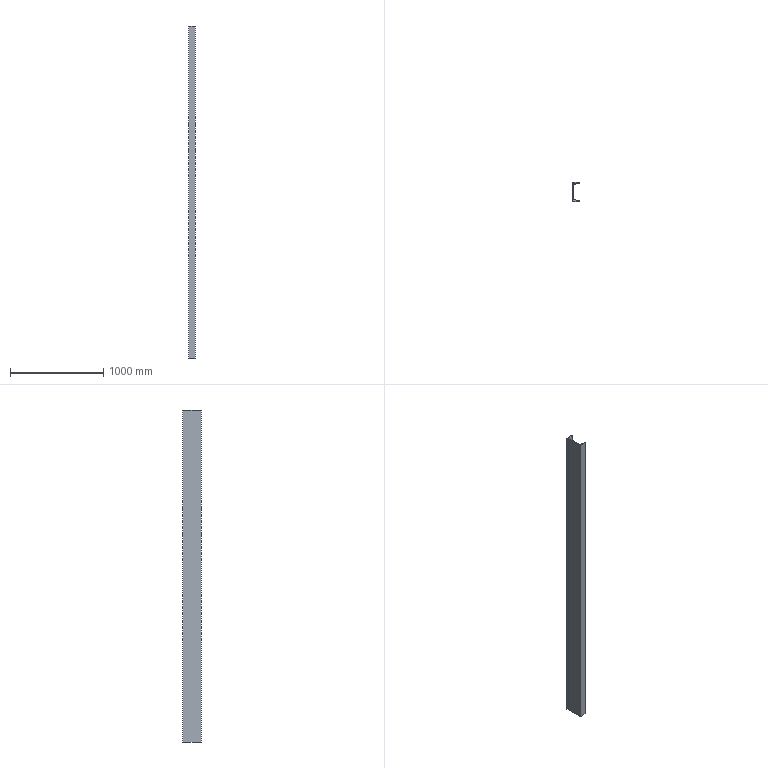Part | SolidWorks | features Extrusion 1 | 1 solid | 14 faces | box 73 x 200 x 3556 mm | volume 10184198 mm3 | plane 10 | cylinder 4 | commonest cylinder face diameters 11 x2 22 x2
STEP:
#1=CARTESIAN_POINT('',(73.,200.,-1778.));
#2=VERTEX_POINT('',#1);
#3=CARTESIAN_POINT('',(0.,200.,-1778.));
#4=VERTEX_POINT('',#3);
#5=CARTESIAN_POINT('',(0.,200.,-1778.));
#6=DIRECTION('',(-1.,0.,0.));
#7=VECTOR('',#6,1000.);
#8=LINE('',#5,#7);
#9=EDGE_CURVE('',#2,#4,#8,.T.);
#10=ORIENTED_EDGE('',*,*,#9,.T.);
#11=CARTESIAN_POINT('',(0.,200.,1778.));
#12=VERTEX_POINT('',#11);
#13=CARTESIAN_POINT('',(0.,200.,1778.));
#14=DIRECTION('',(0.,0.,-1.));
#15=VECTOR('',#14,1000.);
#16=LINE('',#13,#15);
#17=EDGE_CURVE('',#12,#4,#16,.T.);
#18=ORIENTED_EDGE('',*,*,#17,.F.);
#19=CARTESIAN_POINT('',(73.,200.,1778.));
#20=VERTEX_POINT('',#19);
#21=CARTESIAN_POINT('',(0.,200.,1778.));
#22=DIRECTION('',(-1.,0.,0.));
#23=VECTOR('',#22,1000.);
#24=LINE('',#21,#23);
#25=EDGE_CURVE('',#20,#12,#24,.T.);
#26=ORIENTED_EDGE('',*,*,#25,.F.);
#27=CARTESIAN_POINT('',(73.,200.,1778.));
#28=DIRECTION('',(0.,0.,-1.));
#29=VECTOR('',#28,1000.);
#30=LINE('',#27,#29);
#31=EDGE_CURVE('',#20,#2,#30,.T.);
#32=ORIENTED_EDGE('',*,*,#31,.T.);
#33=EDGE_LOOP('',(#10,#18,#26,#32));
#34=FACE_OUTER_BOUND('',#33,.T.);
#35=CARTESIAN_POINT('',(0.,200.,1778.));
#36=DIRECTION('',(0.,-1.,0.));
#37=DIRECTION('',(0.,0.,-1.));
#38=AXIS2_PLACEMENT_3D('',#35,#36,#37);
#39=PLANE('',#38);
#40=ADVANCED_FACE('',(#34),#39,.F.);
#41=CARTESIAN_POINT('',(0.,0.,-1778.));
#42=VERTEX_POINT('',#41);
#43=CARTESIAN_POINT('',(0.,0.,-1778.));
#44=DIRECTION('',(0.,-1.,0.));
#45=VECTOR('',#44,1000.);
#46=LINE('',#43,#45);
#47=EDGE_CURVE('',#4,#42,#46,.T.);
#48=ORIENTED_EDGE('',*,*,#47,.T.);
#49=CARTESIAN_POINT('',(0.,0.,1778.));
#50=VERTEX_POINT('',#49);
#51=CARTESIAN_POINT('',(0.,0.,1778.));
#52=DIRECTION('',(0.,0.,-1.));
#53=VECTOR('',#52,1000.);
#54=LINE('',#51,#53);
#55=EDGE_CURVE('',#50,#42,#54,.T.);
#56=ORIENTED_EDGE('',*,*,#55,.F.);
#57=CARTESIAN_POINT('',(0.,0.,1778.));
#58=DIRECTION('',(0.,-1.,0.));
#59=VECTOR('',#58,1000.);
#60=LINE('',#57,#59);
#61=EDGE_CURVE('',#12,#50,#60,.T.);
#62=ORIENTED_EDGE('',*,*,#61,.F.);
#63=ORIENTED_EDGE('',*,*,#17,.T.);
#64=EDGE_LOOP('',(#48,#56,#62,#63));
#65=FACE_OUTER_BOUND('',#64,.T.);
#66=CARTESIAN_POINT('',(0.,0.,1778.));
#67=DIRECTION('',(1.,0.,0.));
#68=DIRECTION('',(0.,0.,-1.));
#69=AXIS2_PLACEMENT_3D('',#66,#67,#68);
#70=PLANE('',#69);
#71=ADVANCED_FACE('',(#65),#70,.F.);
#72=CARTESIAN_POINT('',(73.,0.,-1778.));
#73=VERTEX_POINT('',#72);
#74=CARTESIAN_POINT('',(0.,0.,-1778.));
#75=DIRECTION('',(1.,0.,0.));
#76=VECTOR('',#75,1000.);
#77=LINE('',#74,#76);
#78=EDGE_CURVE('',#42,#73,#77,.T.);
#79=ORIENTED_EDGE('',*,*,#78,.T.);
#80=CARTESIAN_POINT('',(73.,0.,1778.));
#81=VERTEX_POINT('',#80);
#82=CARTESIAN_POINT('',(73.,0.,1778.));
#83=DIRECTION('',(0.,0.,-1.));
#84=VECTOR('',#83,1000.);
#85=LINE('',#82,#84);
#86=EDGE_CURVE('',#81,#73,#85,.T.);
#87=ORIENTED_EDGE('',*,*,#86,.F.);
#88=CARTESIAN_POINT('',(0.,0.,1778.));
#89=DIRECTION('',(1.,0.,0.));
#90=VECTOR('',#89,1000.);
#91=LINE('',#88,#90);
#92=EDGE_CURVE('',#50,#81,#91,.T.);
#93=ORIENTED_EDGE('',*,*,#92,.F.);
#94=ORIENTED_EDGE('',*,*,#55,.T.);
#95=EDGE_LOOP('',(#79,#87,#93,#94));
#96=FACE_OUTER_BOUND('',#95,.T.);
#97=CARTESIAN_POINT('',(0.,0.,1778.));
#98=DIRECTION('',(0.,1.,0.));
#99=DIRECTION('',(0.,0.,1.));
#100=AXIS2_PLACEMENT_3D('',#97,#98,#99);
#101=PLANE('',#100);
#102=ADVANCED_FACE('',(#96),#101,.F.);
#103=CARTESIAN_POINT('',(73.,3.967,-1778.));
#104=VERTEX_POINT('',#103);
#105=CARTESIAN_POINT('',(73.,3.967,-1778.));
#106=DIRECTION('',(0.,1.,0.));
#107=VECTOR('',#106,1000.);
#108=LINE('',#105,#107);
#109=EDGE_CURVE('',#73,#104,#108,.T.);
#110=ORIENTED_EDGE('',*,*,#109,.T.);
#111=CARTESIAN_POINT('',(73.,3.967,1778.));
#112=VERTEX_POINT('',#111);
#113=CARTESIAN_POINT('',(73.,3.967,1778.));
#114=DIRECTION('',(0.,0.,-1.));
#115=VECTOR('',#114,1000.);
#116=LINE('',#113,#115);
#117=EDGE_CURVE('',#112,#104,#116,.T.);
#118=ORIENTED_EDGE('',*,*,#117,.F.);
#119=CARTESIAN_POINT('',(73.,3.967,1778.));
#120=DIRECTION('',(0.,1.,0.));
#121=VECTOR('',#120,1000.);
#122=LINE('',#119,#121);
#123=EDGE_CURVE('',#81,#112,#122,.T.);
#124=ORIENTED_EDGE('',*,*,#123,.F.);
#125=ORIENTED_EDGE('',*,*,#86,.T.);
#126=EDGE_LOOP('',(#110,#118,#124,#125));
#127=FACE_OUTER_BOUND('',#126,.T.);
#128=CARTESIAN_POINT('',(73.,3.967,1778.));
#129=DIRECTION('',(-1.,0.,0.));
#130=DIRECTION('',(0.,-1.,0.));
#131=AXIS2_PLACEMENT_3D('',#128,#129,#130);
#132=PLANE('',#131);
#133=ADVANCED_FACE('',(#127),#132,.F.);
#134=CARTESIAN_POINT('',(67.771,9.46,-1778.));
#135=VERTEX_POINT('',#134);
#136=CARTESIAN_POINT('',(67.5,3.967,-1778.));
#137=DIRECTION('',(0.,0.,1.));
#138=DIRECTION('',(1.,0.,0.));
#139=AXIS2_PLACEMENT_3D('',#136,#137,#138);
#140=CIRCLE('',#139,5.5);
#141=EDGE_CURVE('',#104,#135,#140,.T.);
#142=ORIENTED_EDGE('',*,*,#141,.T.);
#143=CARTESIAN_POINT('',(67.771,9.46,1778.));
#144=VERTEX_POINT('',#143);
#145=CARTESIAN_POINT('',(67.771,9.46,1778.));
#146=DIRECTION('',(0.,0.,-1.));
#147=VECTOR('',#146,1000.);
#148=LINE('',#145,#147);
#149=EDGE_CURVE('',#144,#135,#148,.T.);
#150=ORIENTED_EDGE('',*,*,#149,.F.);
#151=CARTESIAN_POINT('',(67.5,3.967,1778.));
#152=DIRECTION('',(0.,0.,1.));
#153=DIRECTION('',(1.,0.,0.));
#154=AXIS2_PLACEMENT_3D('',#151,#152,#153);
#155=CIRCLE('',#154,5.5);
#156=EDGE_CURVE('',#112,#144,#155,.T.);
#157=ORIENTED_EDGE('',*,*,#156,.F.);
#158=ORIENTED_EDGE('',*,*,#117,.T.);
#159=EDGE_LOOP('',(#142,#150,#157,#158));
#160=FACE_OUTER_BOUND('',#159,.T.);
#161=CARTESIAN_POINT('',(67.5,3.967,1778.));
#162=DIRECTION('',(0.,0.,-1.));
#163=DIRECTION('',(-1.,0.,0.));
#164=AXIS2_PLACEMENT_3D('',#161,#162,#163);
#165=CYLINDRICAL_SURFACE('',#164,5.5);
#166=ADVANCED_FACE('',(#160),#165,.T.);
#167=CARTESIAN_POINT('',(17.459,11.938,-1778.));
#168=VERTEX_POINT('',#167);
#169=CARTESIAN_POINT('',(17.459,11.938,-1778.));
#170=DIRECTION('',(-0.9988,0.04918,0.));
#171=VECTOR('',#170,1000.);
#172=LINE('',#169,#171);
#173=EDGE_CURVE('',#135,#168,#172,.T.);
#174=ORIENTED_EDGE('',*,*,#173,.T.);
#175=CARTESIAN_POINT('',(17.459,11.938,1778.));
#176=VERTEX_POINT('',#175);
#177=CARTESIAN_POINT('',(17.459,11.938,1778.));
#178=DIRECTION('',(0.,0.,-1.));
#179=VECTOR('',#178,1000.);
#180=LINE('',#177,#179);
#181=EDGE_CURVE('',#176,#168,#180,.T.);
#182=ORIENTED_EDGE('',*,*,#181,.F.);
#183=CARTESIAN_POINT('',(17.459,11.938,1778.));
#184=DIRECTION('',(-0.9988,0.04918,0.));
#185=VECTOR('',#184,1000.);
#186=LINE('',#183,#185);
#187=EDGE_CURVE('',#144,#176,#186,.T.);
#188=ORIENTED_EDGE('',*,*,#187,.F.);
#189=ORIENTED_EDGE('',*,*,#149,.T.);
#190=EDGE_LOOP('',(#174,#182,#188,#189));
#191=FACE_OUTER_BOUND('',#190,.T.);
#192=CARTESIAN_POINT('',(17.459,11.938,1778.));
#193=DIRECTION('',(-0.04918,-0.9988,0.));
#194=DIRECTION('',(0.9988,-0.04918,0.));
#195=AXIS2_PLACEMENT_3D('',#192,#193,#194);
#196=PLANE('',#195);
#197=ADVANCED_FACE('',(#191),#196,.F.);
#198=CARTESIAN_POINT('',(7.,22.924,-1778.));
#199=VERTEX_POINT('',#198);
#200=CARTESIAN_POINT('',(18.,22.924,-1778.));
#201=DIRECTION('',(0.,0.,-1.));
#202=DIRECTION('',(-1.,0.,0.));
#203=AXIS2_PLACEMENT_3D('',#200,#201,#202);
#204=CIRCLE('',#203,11.);
#205=EDGE_CURVE('',#168,#199,#204,.T.);
#206=ORIENTED_EDGE('',*,*,#205,.T.);
#207=CARTESIAN_POINT('',(7.,22.924,1778.));
#208=VERTEX_POINT('',#207);
#209=CARTESIAN_POINT('',(7.,22.924,1778.));
#210=DIRECTION('',(0.,0.,-1.));
#211=VECTOR('',#210,1000.);
#212=LINE('',#209,#211);
#213=EDGE_CURVE('',#208,#199,#212,.T.);
#214=ORIENTED_EDGE('',*,*,#213,.F.);
#215=CARTESIAN_POINT('',(18.,22.924,1778.));
#216=DIRECTION('',(0.,0.,-1.));
#217=DIRECTION('',(-1.,0.,0.));
#218=AXIS2_PLACEMENT_3D('',#215,#216,#217);
#219=CIRCLE('',#218,11.);
#220=EDGE_CURVE('',#176,#208,#219,.T.);
#221=ORIENTED_EDGE('',*,*,#220,.F.);
#222=ORIENTED_EDGE('',*,*,#181,.T.);
#223=EDGE_LOOP('',(#206,#214,#221,#222));
#224=FACE_OUTER_BOUND('',#223,.T.);
#225=CARTESIAN_POINT('',(18.,22.924,1778.));
#226=DIRECTION('',(0.,0.,-1.));
#227=DIRECTION('',(-1.,0.,0.));
#228=AXIS2_PLACEMENT_3D('',#225,#226,#227);
#229=CYLINDRICAL_SURFACE('',#228,11.);
#230=ADVANCED_FACE('',(#224),#229,.F.);
#231=CARTESIAN_POINT('',(7.,177.076,-1778.));
#232=VERTEX_POINT('',#231);
#233=CARTESIAN_POINT('',(7.,177.076,-1778.));
#234=DIRECTION('',(0.,1.,0.));
#235=VECTOR('',#234,1000.);
#236=LINE('',#233,#235);
#237=EDGE_CURVE('',#199,#232,#236,.T.);
#238=ORIENTED_EDGE('',*,*,#237,.T.);
#239=CARTESIAN_POINT('',(7.,177.076,1778.));
#240=VERTEX_POINT('',#239);
#241=CARTESIAN_POINT('',(7.,177.076,1778.));
#242=DIRECTION('',(0.,0.,-1.));
#243=VECTOR('',#242,1000.);
#244=LINE('',#241,#243);
#245=EDGE_CURVE('',#240,#232,#244,.T.);
#246=ORIENTED_EDGE('',*,*,#245,.F.);
#247=CARTESIAN_POINT('',(7.,177.076,1778.));
#248=DIRECTION('',(0.,1.,0.));
#249=VECTOR('',#248,1000.);
#250=LINE('',#247,#249);
#251=EDGE_CURVE('',#208,#240,#250,.T.);
#252=ORIENTED_EDGE('',*,*,#251,.F.);
#253=ORIENTED_EDGE('',*,*,#213,.T.);
#254=EDGE_LOOP('',(#238,#246,#252,#253));
#255=FACE_OUTER_BOUND('',#254,.T.);
#256=CARTESIAN_POINT('',(7.,177.076,1778.));
#257=DIRECTION('',(-1.,0.,0.));
#258=DIRECTION('',(0.,0.,1.));
#259=AXIS2_PLACEMENT_3D('',#256,#257,#258);
#260=PLANE('',#259);
#261=ADVANCED_FACE('',(#255),#260,.F.);
#262=CARTESIAN_POINT('',(17.459,188.062,-1778.));
#263=VERTEX_POINT('',#262);
#264=CARTESIAN_POINT('',(18.,177.076,-1778.));
#265=DIRECTION('',(0.,0.,-1.));
#266=DIRECTION('',(-1.,0.,0.));
#267=AXIS2_PLACEMENT_3D('',#264,#265,#266);
#268=CIRCLE('',#267,11.);
#269=EDGE_CURVE('',#232,#263,#268,.T.);
#270=ORIENTED_EDGE('',*,*,#269,.T.);
#271=CARTESIAN_POINT('',(17.459,188.062,1778.));
#272=VERTEX_POINT('',#271);
#273=CARTESIAN_POINT('',(17.459,188.062,1778.));
#274=DIRECTION('',(0.,0.,-1.));
#275=VECTOR('',#274,1000.);
#276=LINE('',#273,#275);
#277=EDGE_CURVE('',#272,#263,#276,.T.);
#278=ORIENTED_EDGE('',*,*,#277,.F.);
#279=CARTESIAN_POINT('',(18.,177.076,1778.));
#280=DIRECTION('',(0.,0.,-1.));
#281=DIRECTION('',(-1.,0.,0.));
#282=AXIS2_PLACEMENT_3D('',#279,#280,#281);
#283=CIRCLE('',#282,11.);
#284=EDGE_CURVE('',#240,#272,#283,.T.);
#285=ORIENTED_EDGE('',*,*,#284,.F.);
#286=ORIENTED_EDGE('',*,*,#245,.T.);
#287=EDGE_LOOP('',(#270,#278,#285,#286));
#288=FACE_OUTER_BOUND('',#287,.T.);
#289=CARTESIAN_POINT('',(18.,177.076,1778.));
#290=DIRECTION('',(0.,0.,-1.));
#291=DIRECTION('',(-1.,0.,0.));
#292=AXIS2_PLACEMENT_3D('',#289,#290,#291);
#293=CYLINDRICAL_SURFACE('',#292,11.);
#294=ADVANCED_FACE('',(#288),#293,.F.);
#295=CARTESIAN_POINT('',(67.771,190.54,-1778.));
#296=VERTEX_POINT('',#295);
#297=CARTESIAN_POINT('',(17.459,188.062,-1778.));
#298=DIRECTION('',(0.9988,0.04918,0.));
#299=VECTOR('',#298,1000.);
#300=LINE('',#297,#299);
#301=EDGE_CURVE('',#263,#296,#300,.T.);
#302=ORIENTED_EDGE('',*,*,#301,.T.);
#303=CARTESIAN_POINT('',(67.771,190.54,1778.));
#304=VERTEX_POINT('',#303);
#305=CARTESIAN_POINT('',(67.771,190.54,1778.));
#306=DIRECTION('',(0.,0.,-1.));
#307=VECTOR('',#306,1000.);
#308=LINE('',#305,#307);
#309=EDGE_CURVE('',#304,#296,#308,.T.);
#310=ORIENTED_EDGE('',*,*,#309,.F.);
#311=CARTESIAN_POINT('',(17.459,188.062,1778.));
#312=DIRECTION('',(0.9988,0.04918,0.));
#313=VECTOR('',#312,1000.);
#314=LINE('',#311,#313);
#315=EDGE_CURVE('',#272,#304,#314,.T.);
#316=ORIENTED_EDGE('',*,*,#315,.F.);
#317=ORIENTED_EDGE('',*,*,#277,.T.);
#318=EDGE_LOOP('',(#302,#310,#316,#317));
#319=FACE_OUTER_BOUND('',#318,.T.);
#320=CARTESIAN_POINT('',(17.459,188.062,1778.));
#321=DIRECTION('',(-0.04918,0.9988,0.));
#322=DIRECTION('',(-0.9988,-0.04918,0.));
#323=AXIS2_PLACEMENT_3D('',#320,#321,#322);
#324=PLANE('',#323);
#325=ADVANCED_FACE('',(#319),#324,.F.);
#326=CARTESIAN_POINT('',(73.,196.033,-1778.));
#327=VERTEX_POINT('',#326);
#328=CARTESIAN_POINT('',(67.5,196.033,-1778.));
#329=DIRECTION('',(0.,0.,1.));
#330=DIRECTION('',(1.,0.,0.));
#331=AXIS2_PLACEMENT_3D('',#328,#329,#330);
#332=CIRCLE('',#331,5.5);
#333=EDGE_CURVE('',#296,#327,#332,.T.);
#334=ORIENTED_EDGE('',*,*,#333,.T.);
#335=CARTESIAN_POINT('',(73.,196.033,1778.));
#336=VERTEX_POINT('',#335);
#337=CARTESIAN_POINT('',(73.,196.033,1778.));
#338=DIRECTION('',(0.,0.,-1.));
#339=VECTOR('',#338,1000.);
#340=LINE('',#337,#339);
#341=EDGE_CURVE('',#336,#327,#340,.T.);
#342=ORIENTED_EDGE('',*,*,#341,.F.);
#343=CARTESIAN_POINT('',(67.5,196.033,1778.));
#344=DIRECTION('',(0.,0.,1.));
#345=DIRECTION('',(1.,0.,0.));
#346=AXIS2_PLACEMENT_3D('',#343,#344,#345);
#347=CIRCLE('',#346,5.5);
#348=EDGE_CURVE('',#304,#336,#347,.T.);
#349=ORIENTED_EDGE('',*,*,#348,.F.);
#350=ORIENTED_EDGE('',*,*,#309,.T.);
#351=EDGE_LOOP('',(#334,#342,#349,#350));
#352=FACE_OUTER_BOUND('',#351,.T.);
#353=CARTESIAN_POINT('',(67.5,196.033,1778.));
#354=DIRECTION('',(0.,0.,-1.));
#355=DIRECTION('',(-1.,0.,0.));
#356=AXIS2_PLACEMENT_3D('',#353,#354,#355);
#357=CYLINDRICAL_SURFACE('',#356,5.5);
#358=ADVANCED_FACE('',(#352),#357,.T.);
#359=CARTESIAN_POINT('',(73.,196.033,-1778.));
#360=DIRECTION('',(0.,1.,0.));
#361=VECTOR('',#360,1000.);
#362=LINE('',#359,#361);
#363=EDGE_CURVE('',#327,#2,#362,.T.);
#364=ORIENTED_EDGE('',*,*,#363,.T.);
#365=ORIENTED_EDGE('',*,*,#31,.F.);
#366=CARTESIAN_POINT('',(73.,196.033,1778.));
#367=DIRECTION('',(0.,1.,0.));
#368=VECTOR('',#367,1000.);
#369=LINE('',#366,#368);
#370=EDGE_CURVE('',#336,#20,#369,.T.);
#371=ORIENTED_EDGE('',*,*,#370,.F.);
#372=ORIENTED_EDGE('',*,*,#341,.T.);
#373=EDGE_LOOP('',(#364,#365,#371,#372));
#374=FACE_OUTER_BOUND('',#373,.T.);
#375=CARTESIAN_POINT('',(73.,196.033,1778.));
#376=DIRECTION('',(-1.,0.,0.));
#377=DIRECTION('',(0.,-1.,0.));
#378=AXIS2_PLACEMENT_3D('',#375,#376,#377);
#379=PLANE('',#378);
#380=ADVANCED_FACE('',(#374),#379,.F.);
#381=ORIENTED_EDGE('',*,*,#25,.T.);
#382=ORIENTED_EDGE('',*,*,#61,.T.);
#383=ORIENTED_EDGE('',*,*,#92,.T.);
#384=ORIENTED_EDGE('',*,*,#123,.T.);
#385=ORIENTED_EDGE('',*,*,#156,.T.);
#386=ORIENTED_EDGE('',*,*,#187,.T.);
#387=ORIENTED_EDGE('',*,*,#220,.T.);
#388=ORIENTED_EDGE('',*,*,#251,.T.);
#389=ORIENTED_EDGE('',*,*,#284,.T.);
#390=ORIENTED_EDGE('',*,*,#315,.T.);
#391=ORIENTED_EDGE('',*,*,#348,.T.);
#392=ORIENTED_EDGE('',*,*,#370,.T.);
#393=EDGE_LOOP('',(#381,#382,#383,#384,#385,#386,#387,#388,#389,#390,#391,#392));
#394=FACE_OUTER_BOUND('',#393,.T.);
#395=CARTESIAN_POINT('',(67.5,196.033,1778.));
#396=DIRECTION('',(0.,0.,1.));
#397=DIRECTION('',(1.,0.,0.));
#398=AXIS2_PLACEMENT_3D('',#395,#396,#397);
#399=PLANE('',#398);
#400=ADVANCED_FACE('',(#394),#399,.T.);
#401=ORIENTED_EDGE('',*,*,#9,.F.);
#402=ORIENTED_EDGE('',*,*,#363,.F.);
#403=ORIENTED_EDGE('',*,*,#333,.F.);
#404=ORIENTED_EDGE('',*,*,#301,.F.);
#405=ORIENTED_EDGE('',*,*,#269,.F.);
#406=ORIENTED_EDGE('',*,*,#237,.F.);
#407=ORIENTED_EDGE('',*,*,#205,.F.);
#408=ORIENTED_EDGE('',*,*,#173,.F.);
#409=ORIENTED_EDGE('',*,*,#141,.F.);
#410=ORIENTED_EDGE('',*,*,#109,.F.);
#411=ORIENTED_EDGE('',*,*,#78,.F.);
#412=ORIENTED_EDGE('',*,*,#47,.F.);
#413=EDGE_LOOP('',(#401,#402,#403,#404,#405,#406,#407,#408,#409,#410,#411,#412));
#414=FACE_OUTER_BOUND('',#413,.T.);
#415=CARTESIAN_POINT('',(67.5,196.033,-1778.));
#416=DIRECTION('',(0.,0.,1.));
#417=DIRECTION('',(1.,0.,0.));
#418=AXIS2_PLACEMENT_3D('',#415,#416,#417);
#419=PLANE('',#418);
#420=ADVANCED_FACE('',(#414),#419,.F.);
#421=CLOSED_SHELL('',(#40,#71,#102,#133,#166,#197,#230,#261,#294,#325,#358,#380,#400,#420));
#422=MANIFOLD_SOLID_BREP('',#421);
#423=CARTESIAN_POINT('',(0.,0.,0.));
#424=DIRECTION('',(0.,0.,1.));
#425=DIRECTION('',(1.,0.,0.));
#426=AXIS2_PLACEMENT_3D('',#423,#424,#425);
#427=(LENGTH_UNIT()NAMED_UNIT(*)SI_UNIT(.MILLI.,.METRE.));
#428=UNCERTAINTY_MEASURE_WITH_UNIT(LENGTH_MEASURE(0.00001),#427,'','');
#429=(NAMED_UNIT(*)PLANE_ANGLE_UNIT()SI_UNIT($,.RADIAN.));
#430=(NAMED_UNIT(*)SI_UNIT($,.STERADIAN.)SOLID_ANGLE_UNIT());
#431=(GEOMETRIC_REPRESENTATION_CONTEXT(3)GLOBAL_UNCERTAINTY_ASSIGNED_CONTEXT((#428))GLOBAL_UNIT_ASSIGNED_CONTEXT((#427,#429,#430))REPRESENTATION_CONTEXT('',''));
#432=ADVANCED_BREP_SHAPE_REPRESENTATION('',(#422,#426),#431);